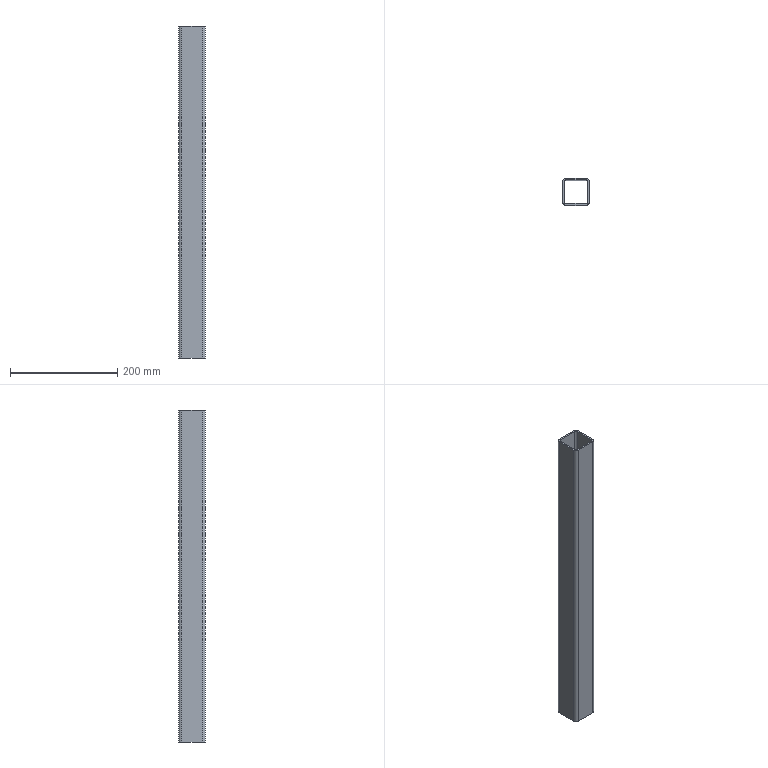Part | SolidWorks | 1 solid | 18 faces | box 50 x 50 x 620 mm | volume 335310 mm3 | plane 10 | cylinder 8 | commonest cylinder face diameters 6 x4 12 x4
STEP:
#1=CARTESIAN_POINT('',(19.,25.,310.));
#2=VERTEX_POINT('',#1);
#3=CARTESIAN_POINT('',(25.,19.,310.));
#4=VERTEX_POINT('',#3);
#5=CARTESIAN_POINT('',(19.,19.,310.));
#6=DIRECTION('',(0.,0.,-1.));
#7=DIRECTION('',(-1.,0.,0.));
#8=AXIS2_PLACEMENT_3D('',#5,#6,#7);
#9=CIRCLE('',#8,6.);
#10=EDGE_CURVE('',#2,#4,#9,.T.);
#11=ORIENTED_EDGE('',*,*,#10,.T.);
#12=CARTESIAN_POINT('',(25.,19.,-310.));
#13=VERTEX_POINT('',#12);
#14=CARTESIAN_POINT('',(25.,19.,-310.));
#15=DIRECTION('',(0.,0.,1.));
#16=VECTOR('',#15,1000.);
#17=LINE('',#14,#16);
#18=EDGE_CURVE('',#13,#4,#17,.T.);
#19=ORIENTED_EDGE('',*,*,#18,.F.);
#20=CARTESIAN_POINT('',(19.,25.,-310.));
#21=VERTEX_POINT('',#20);
#22=CARTESIAN_POINT('',(19.,19.,-310.));
#23=DIRECTION('',(0.,0.,-1.));
#24=DIRECTION('',(-1.,0.,0.));
#25=AXIS2_PLACEMENT_3D('',#22,#23,#24);
#26=CIRCLE('',#25,6.);
#27=EDGE_CURVE('',#21,#13,#26,.T.);
#28=ORIENTED_EDGE('',*,*,#27,.F.);
#29=CARTESIAN_POINT('',(19.,25.,-310.));
#30=DIRECTION('',(0.,0.,1.));
#31=VECTOR('',#30,1000.);
#32=LINE('',#29,#31);
#33=EDGE_CURVE('',#21,#2,#32,.T.);
#34=ORIENTED_EDGE('',*,*,#33,.T.);
#35=EDGE_LOOP('',(#11,#19,#28,#34));
#36=FACE_OUTER_BOUND('',#35,.T.);
#37=CARTESIAN_POINT('',(19.,19.,-310.));
#38=DIRECTION('',(0.,0.,1.));
#39=DIRECTION('',(1.,0.,0.));
#40=AXIS2_PLACEMENT_3D('',#37,#38,#39);
#41=CYLINDRICAL_SURFACE('',#40,6.);
#42=ADVANCED_FACE('',(#36),#41,.T.);
#43=CARTESIAN_POINT('',(25.,-19.,310.));
#44=VERTEX_POINT('',#43);
#45=CARTESIAN_POINT('',(25.,19.,310.));
#46=DIRECTION('',(0.,-1.,0.));
#47=VECTOR('',#46,1000.);
#48=LINE('',#45,#47);
#49=EDGE_CURVE('',#4,#44,#48,.T.);
#50=ORIENTED_EDGE('',*,*,#49,.T.);
#51=CARTESIAN_POINT('',(25.,-19.,-310.));
#52=VERTEX_POINT('',#51);
#53=CARTESIAN_POINT('',(25.,-19.,-310.));
#54=DIRECTION('',(0.,0.,1.));
#55=VECTOR('',#54,1000.);
#56=LINE('',#53,#55);
#57=EDGE_CURVE('',#52,#44,#56,.T.);
#58=ORIENTED_EDGE('',*,*,#57,.F.);
#59=CARTESIAN_POINT('',(25.,19.,-310.));
#60=DIRECTION('',(0.,-1.,0.));
#61=VECTOR('',#60,1000.);
#62=LINE('',#59,#61);
#63=EDGE_CURVE('',#13,#52,#62,.T.);
#64=ORIENTED_EDGE('',*,*,#63,.F.);
#65=ORIENTED_EDGE('',*,*,#18,.T.);
#66=EDGE_LOOP('',(#50,#58,#64,#65));
#67=FACE_OUTER_BOUND('',#66,.T.);
#68=CARTESIAN_POINT('',(25.,19.,-310.));
#69=DIRECTION('',(-1.,0.,0.));
#70=DIRECTION('',(0.,0.,1.));
#71=AXIS2_PLACEMENT_3D('',#68,#69,#70);
#72=PLANE('',#71);
#73=ADVANCED_FACE('',(#67),#72,.F.);
#74=CARTESIAN_POINT('',(19.,-25.,310.));
#75=VERTEX_POINT('',#74);
#76=CARTESIAN_POINT('',(19.,-19.,310.));
#77=DIRECTION('',(0.,0.,-1.));
#78=DIRECTION('',(-1.,0.,0.));
#79=AXIS2_PLACEMENT_3D('',#76,#77,#78);
#80=CIRCLE('',#79,6.);
#81=EDGE_CURVE('',#44,#75,#80,.T.);
#82=ORIENTED_EDGE('',*,*,#81,.T.);
#83=CARTESIAN_POINT('',(19.,-25.,-310.));
#84=VERTEX_POINT('',#83);
#85=CARTESIAN_POINT('',(19.,-25.,-310.));
#86=DIRECTION('',(0.,0.,1.));
#87=VECTOR('',#86,1000.);
#88=LINE('',#85,#87);
#89=EDGE_CURVE('',#84,#75,#88,.T.);
#90=ORIENTED_EDGE('',*,*,#89,.F.);
#91=CARTESIAN_POINT('',(19.,-19.,-310.));
#92=DIRECTION('',(0.,0.,-1.));
#93=DIRECTION('',(-1.,0.,0.));
#94=AXIS2_PLACEMENT_3D('',#91,#92,#93);
#95=CIRCLE('',#94,6.);
#96=EDGE_CURVE('',#52,#84,#95,.T.);
#97=ORIENTED_EDGE('',*,*,#96,.F.);
#98=ORIENTED_EDGE('',*,*,#57,.T.);
#99=EDGE_LOOP('',(#82,#90,#97,#98));
#100=FACE_OUTER_BOUND('',#99,.T.);
#101=CARTESIAN_POINT('',(19.,-19.,-310.));
#102=DIRECTION('',(0.,0.,1.));
#103=DIRECTION('',(1.,0.,0.));
#104=AXIS2_PLACEMENT_3D('',#101,#102,#103);
#105=CYLINDRICAL_SURFACE('',#104,6.);
#106=ADVANCED_FACE('',(#100),#105,.T.);
#107=CARTESIAN_POINT('',(-19.,-25.,310.));
#108=VERTEX_POINT('',#107);
#109=CARTESIAN_POINT('',(-19.,-25.,310.));
#110=DIRECTION('',(-1.,0.,0.));
#111=VECTOR('',#110,1000.);
#112=LINE('',#109,#111);
#113=EDGE_CURVE('',#75,#108,#112,.T.);
#114=ORIENTED_EDGE('',*,*,#113,.T.);
#115=CARTESIAN_POINT('',(-19.,-25.,-310.));
#116=VERTEX_POINT('',#115);
#117=CARTESIAN_POINT('',(-19.,-25.,-310.));
#118=DIRECTION('',(0.,0.,1.));
#119=VECTOR('',#118,1000.);
#120=LINE('',#117,#119);
#121=EDGE_CURVE('',#116,#108,#120,.T.);
#122=ORIENTED_EDGE('',*,*,#121,.F.);
#123=CARTESIAN_POINT('',(-19.,-25.,-310.));
#124=DIRECTION('',(-1.,0.,0.));
#125=VECTOR('',#124,1000.);
#126=LINE('',#123,#125);
#127=EDGE_CURVE('',#84,#116,#126,.T.);
#128=ORIENTED_EDGE('',*,*,#127,.F.);
#129=ORIENTED_EDGE('',*,*,#89,.T.);
#130=EDGE_LOOP('',(#114,#122,#128,#129));
#131=FACE_OUTER_BOUND('',#130,.T.);
#132=CARTESIAN_POINT('',(-19.,-25.,-310.));
#133=DIRECTION('',(0.,1.,0.));
#134=DIRECTION('',(0.,0.,1.));
#135=AXIS2_PLACEMENT_3D('',#132,#133,#134);
#136=PLANE('',#135);
#137=ADVANCED_FACE('',(#131),#136,.F.);
#138=CARTESIAN_POINT('',(-25.,-19.,310.));
#139=VERTEX_POINT('',#138);
#140=CARTESIAN_POINT('',(-19.,-19.,310.));
#141=DIRECTION('',(0.,0.,-1.));
#142=DIRECTION('',(-1.,0.,0.));
#143=AXIS2_PLACEMENT_3D('',#140,#141,#142);
#144=CIRCLE('',#143,6.);
#145=EDGE_CURVE('',#108,#139,#144,.T.);
#146=ORIENTED_EDGE('',*,*,#145,.T.);
#147=CARTESIAN_POINT('',(-25.,-19.,-310.));
#148=VERTEX_POINT('',#147);
#149=CARTESIAN_POINT('',(-25.,-19.,-310.));
#150=DIRECTION('',(0.,0.,1.));
#151=VECTOR('',#150,1000.);
#152=LINE('',#149,#151);
#153=EDGE_CURVE('',#148,#139,#152,.T.);
#154=ORIENTED_EDGE('',*,*,#153,.F.);
#155=CARTESIAN_POINT('',(-19.,-19.,-310.));
#156=DIRECTION('',(0.,0.,-1.));
#157=DIRECTION('',(-1.,0.,0.));
#158=AXIS2_PLACEMENT_3D('',#155,#156,#157);
#159=CIRCLE('',#158,6.);
#160=EDGE_CURVE('',#116,#148,#159,.T.);
#161=ORIENTED_EDGE('',*,*,#160,.F.);
#162=ORIENTED_EDGE('',*,*,#121,.T.);
#163=EDGE_LOOP('',(#146,#154,#161,#162));
#164=FACE_OUTER_BOUND('',#163,.T.);
#165=CARTESIAN_POINT('',(-19.,-19.,-310.));
#166=DIRECTION('',(0.,0.,1.));
#167=DIRECTION('',(1.,0.,0.));
#168=AXIS2_PLACEMENT_3D('',#165,#166,#167);
#169=CYLINDRICAL_SURFACE('',#168,6.);
#170=ADVANCED_FACE('',(#164),#169,.T.);
#171=CARTESIAN_POINT('',(-25.,19.,310.));
#172=VERTEX_POINT('',#171);
#173=CARTESIAN_POINT('',(-25.,-19.,310.));
#174=DIRECTION('',(0.,1.,0.));
#175=VECTOR('',#174,1000.);
#176=LINE('',#173,#175);
#177=EDGE_CURVE('',#139,#172,#176,.T.);
#178=ORIENTED_EDGE('',*,*,#177,.T.);
#179=CARTESIAN_POINT('',(-25.,19.,-310.));
#180=VERTEX_POINT('',#179);
#181=CARTESIAN_POINT('',(-25.,19.,-310.));
#182=DIRECTION('',(0.,0.,1.));
#183=VECTOR('',#182,1000.);
#184=LINE('',#181,#183);
#185=EDGE_CURVE('',#180,#172,#184,.T.);
#186=ORIENTED_EDGE('',*,*,#185,.F.);
#187=CARTESIAN_POINT('',(-25.,-19.,-310.));
#188=DIRECTION('',(0.,1.,0.));
#189=VECTOR('',#188,1000.);
#190=LINE('',#187,#189);
#191=EDGE_CURVE('',#148,#180,#190,.T.);
#192=ORIENTED_EDGE('',*,*,#191,.F.);
#193=ORIENTED_EDGE('',*,*,#153,.T.);
#194=EDGE_LOOP('',(#178,#186,#192,#193));
#195=FACE_OUTER_BOUND('',#194,.T.);
#196=CARTESIAN_POINT('',(-25.,-19.,-310.));
#197=DIRECTION('',(1.,0.,0.));
#198=DIRECTION('',(0.,0.,-1.));
#199=AXIS2_PLACEMENT_3D('',#196,#197,#198);
#200=PLANE('',#199);
#201=ADVANCED_FACE('',(#195),#200,.F.);
#202=CARTESIAN_POINT('',(-19.,25.,310.));
#203=VERTEX_POINT('',#202);
#204=CARTESIAN_POINT('',(-19.,19.,310.));
#205=DIRECTION('',(0.,0.,-1.));
#206=DIRECTION('',(-1.,0.,0.));
#207=AXIS2_PLACEMENT_3D('',#204,#205,#206);
#208=CIRCLE('',#207,6.);
#209=EDGE_CURVE('',#172,#203,#208,.T.);
#210=ORIENTED_EDGE('',*,*,#209,.T.);
#211=CARTESIAN_POINT('',(-19.,25.,-310.));
#212=VERTEX_POINT('',#211);
#213=CARTESIAN_POINT('',(-19.,25.,-310.));
#214=DIRECTION('',(0.,0.,1.));
#215=VECTOR('',#214,1000.);
#216=LINE('',#213,#215);
#217=EDGE_CURVE('',#212,#203,#216,.T.);
#218=ORIENTED_EDGE('',*,*,#217,.F.);
#219=CARTESIAN_POINT('',(-19.,19.,-310.));
#220=DIRECTION('',(0.,0.,-1.));
#221=DIRECTION('',(-1.,0.,0.));
#222=AXIS2_PLACEMENT_3D('',#219,#220,#221);
#223=CIRCLE('',#222,6.);
#224=EDGE_CURVE('',#180,#212,#223,.T.);
#225=ORIENTED_EDGE('',*,*,#224,.F.);
#226=ORIENTED_EDGE('',*,*,#185,.T.);
#227=EDGE_LOOP('',(#210,#218,#225,#226));
#228=FACE_OUTER_BOUND('',#227,.T.);
#229=CARTESIAN_POINT('',(-19.,19.,-310.));
#230=DIRECTION('',(0.,0.,1.));
#231=DIRECTION('',(1.,0.,0.));
#232=AXIS2_PLACEMENT_3D('',#229,#230,#231);
#233=CYLINDRICAL_SURFACE('',#232,6.);
#234=ADVANCED_FACE('',(#228),#233,.T.);
#235=CARTESIAN_POINT('',(22.,-19.,310.));
#236=VERTEX_POINT('',#235);
#237=CARTESIAN_POINT('',(19.,-22.,310.));
#238=VERTEX_POINT('',#237);
#239=CARTESIAN_POINT('',(19.,-19.,310.));
#240=DIRECTION('',(0.,0.,-1.));
#241=DIRECTION('',(-1.,0.,0.));
#242=AXIS2_PLACEMENT_3D('',#239,#240,#241);
#243=CIRCLE('',#242,3.);
#244=EDGE_CURVE('',#236,#238,#243,.T.);
#245=ORIENTED_EDGE('',*,*,#244,.F.);
#246=CARTESIAN_POINT('',(22.,-19.,-310.));
#247=VERTEX_POINT('',#246);
#248=CARTESIAN_POINT('',(22.,-19.,-310.));
#249=DIRECTION('',(0.,0.,1.));
#250=VECTOR('',#249,1000.);
#251=LINE('',#248,#250);
#252=EDGE_CURVE('',#247,#236,#251,.T.);
#253=ORIENTED_EDGE('',*,*,#252,.F.);
#254=CARTESIAN_POINT('',(19.,-22.,-310.));
#255=VERTEX_POINT('',#254);
#256=CARTESIAN_POINT('',(19.,-19.,-310.));
#257=DIRECTION('',(0.,0.,-1.));
#258=DIRECTION('',(-1.,0.,0.));
#259=AXIS2_PLACEMENT_3D('',#256,#257,#258);
#260=CIRCLE('',#259,3.);
#261=EDGE_CURVE('',#247,#255,#260,.T.);
#262=ORIENTED_EDGE('',*,*,#261,.T.);
#263=CARTESIAN_POINT('',(19.,-22.,-310.));
#264=DIRECTION('',(0.,0.,1.));
#265=VECTOR('',#264,1000.);
#266=LINE('',#263,#265);
#267=EDGE_CURVE('',#255,#238,#266,.T.);
#268=ORIENTED_EDGE('',*,*,#267,.T.);
#269=EDGE_LOOP('',(#245,#253,#262,#268));
#270=FACE_OUTER_BOUND('',#269,.T.);
#271=CARTESIAN_POINT('',(19.,-19.,-310.));
#272=DIRECTION('',(0.,0.,1.));
#273=DIRECTION('',(1.,0.,0.));
#274=AXIS2_PLACEMENT_3D('',#271,#272,#273);
#275=CYLINDRICAL_SURFACE('',#274,3.);
#276=ADVANCED_FACE('',(#270),#275,.F.);
#277=CARTESIAN_POINT('',(22.,19.,310.));
#278=VERTEX_POINT('',#277);
#279=CARTESIAN_POINT('',(22.,19.,310.));
#280=DIRECTION('',(0.,-1.,0.));
#281=VECTOR('',#280,1000.);
#282=LINE('',#279,#281);
#283=EDGE_CURVE('',#278,#236,#282,.T.);
#284=ORIENTED_EDGE('',*,*,#283,.F.);
#285=CARTESIAN_POINT('',(22.,19.,-310.));
#286=VERTEX_POINT('',#285);
#287=CARTESIAN_POINT('',(22.,19.,-310.));
#288=DIRECTION('',(0.,0.,1.));
#289=VECTOR('',#288,1000.);
#290=LINE('',#287,#289);
#291=EDGE_CURVE('',#286,#278,#290,.T.);
#292=ORIENTED_EDGE('',*,*,#291,.F.);
#293=CARTESIAN_POINT('',(22.,19.,-310.));
#294=DIRECTION('',(0.,-1.,0.));
#295=VECTOR('',#294,1000.);
#296=LINE('',#293,#295);
#297=EDGE_CURVE('',#286,#247,#296,.T.);
#298=ORIENTED_EDGE('',*,*,#297,.T.);
#299=ORIENTED_EDGE('',*,*,#252,.T.);
#300=EDGE_LOOP('',(#284,#292,#298,#299));
#301=FACE_OUTER_BOUND('',#300,.T.);
#302=CARTESIAN_POINT('',(22.,19.,-310.));
#303=DIRECTION('',(-1.,0.,0.));
#304=DIRECTION('',(0.,0.,1.));
#305=AXIS2_PLACEMENT_3D('',#302,#303,#304);
#306=PLANE('',#305);
#307=ADVANCED_FACE('',(#301),#306,.T.);
#308=CARTESIAN_POINT('',(19.,22.,310.));
#309=VERTEX_POINT('',#308);
#310=CARTESIAN_POINT('',(19.,19.,310.));
#311=DIRECTION('',(0.,0.,-1.));
#312=DIRECTION('',(-1.,0.,0.));
#313=AXIS2_PLACEMENT_3D('',#310,#311,#312);
#314=CIRCLE('',#313,3.);
#315=EDGE_CURVE('',#309,#278,#314,.T.);
#316=ORIENTED_EDGE('',*,*,#315,.F.);
#317=CARTESIAN_POINT('',(19.,22.,-310.));
#318=VERTEX_POINT('',#317);
#319=CARTESIAN_POINT('',(19.,22.,-310.));
#320=DIRECTION('',(0.,0.,1.));
#321=VECTOR('',#320,1000.);
#322=LINE('',#319,#321);
#323=EDGE_CURVE('',#318,#309,#322,.T.);
#324=ORIENTED_EDGE('',*,*,#323,.F.);
#325=CARTESIAN_POINT('',(19.,19.,-310.));
#326=DIRECTION('',(0.,0.,-1.));
#327=DIRECTION('',(-1.,0.,0.));
#328=AXIS2_PLACEMENT_3D('',#325,#326,#327);
#329=CIRCLE('',#328,3.);
#330=EDGE_CURVE('',#318,#286,#329,.T.);
#331=ORIENTED_EDGE('',*,*,#330,.T.);
#332=ORIENTED_EDGE('',*,*,#291,.T.);
#333=EDGE_LOOP('',(#316,#324,#331,#332));
#334=FACE_OUTER_BOUND('',#333,.T.);
#335=CARTESIAN_POINT('',(19.,19.,-310.));
#336=DIRECTION('',(0.,0.,1.));
#337=DIRECTION('',(1.,0.,0.));
#338=AXIS2_PLACEMENT_3D('',#335,#336,#337);
#339=CYLINDRICAL_SURFACE('',#338,3.);
#340=ADVANCED_FACE('',(#334),#339,.F.);
#341=CARTESIAN_POINT('',(-19.,22.,310.));
#342=VERTEX_POINT('',#341);
#343=CARTESIAN_POINT('',(19.,22.,310.));
#344=DIRECTION('',(1.,0.,0.));
#345=VECTOR('',#344,1000.);
#346=LINE('',#343,#345);
#347=EDGE_CURVE('',#342,#309,#346,.T.);
#348=ORIENTED_EDGE('',*,*,#347,.F.);
#349=CARTESIAN_POINT('',(-19.,22.,-310.));
#350=VERTEX_POINT('',#349);
#351=CARTESIAN_POINT('',(-19.,22.,-310.));
#352=DIRECTION('',(0.,0.,1.));
#353=VECTOR('',#352,1000.);
#354=LINE('',#351,#353);
#355=EDGE_CURVE('',#350,#342,#354,.T.);
#356=ORIENTED_EDGE('',*,*,#355,.F.);
#357=CARTESIAN_POINT('',(19.,22.,-310.));
#358=DIRECTION('',(1.,0.,0.));
#359=VECTOR('',#358,1000.);
#360=LINE('',#357,#359);
#361=EDGE_CURVE('',#350,#318,#360,.T.);
#362=ORIENTED_EDGE('',*,*,#361,.T.);
#363=ORIENTED_EDGE('',*,*,#323,.T.);
#364=EDGE_LOOP('',(#348,#356,#362,#363));
#365=FACE_OUTER_BOUND('',#364,.T.);
#366=CARTESIAN_POINT('',(19.,22.,-310.));
#367=DIRECTION('',(0.,-1.,0.));
#368=DIRECTION('',(0.,0.,-1.));
#369=AXIS2_PLACEMENT_3D('',#366,#367,#368);
#370=PLANE('',#369);
#371=ADVANCED_FACE('',(#365),#370,.T.);
#372=CARTESIAN_POINT('',(-22.,19.,310.));
#373=VERTEX_POINT('',#372);
#374=CARTESIAN_POINT('',(-19.,19.,310.));
#375=DIRECTION('',(0.,0.,-1.));
#376=DIRECTION('',(-1.,0.,0.));
#377=AXIS2_PLACEMENT_3D('',#374,#375,#376);
#378=CIRCLE('',#377,3.);
#379=EDGE_CURVE('',#373,#342,#378,.T.);
#380=ORIENTED_EDGE('',*,*,#379,.F.);
#381=CARTESIAN_POINT('',(-22.,19.,-310.));
#382=VERTEX_POINT('',#381);
#383=CARTESIAN_POINT('',(-22.,19.,-310.));
#384=DIRECTION('',(0.,0.,1.));
#385=VECTOR('',#384,1000.);
#386=LINE('',#383,#385);
#387=EDGE_CURVE('',#382,#373,#386,.T.);
#388=ORIENTED_EDGE('',*,*,#387,.F.);
#389=CARTESIAN_POINT('',(-19.,19.,-310.));
#390=DIRECTION('',(0.,0.,-1.));
#391=DIRECTION('',(-1.,0.,0.));
#392=AXIS2_PLACEMENT_3D('',#389,#390,#391);
#393=CIRCLE('',#392,3.);
#394=EDGE_CURVE('',#382,#350,#393,.T.);
#395=ORIENTED_EDGE('',*,*,#394,.T.);
#396=ORIENTED_EDGE('',*,*,#355,.T.);
#397=EDGE_LOOP('',(#380,#388,#395,#396));
#398=FACE_OUTER_BOUND('',#397,.T.);
#399=CARTESIAN_POINT('',(-19.,19.,-310.));
#400=DIRECTION('',(0.,0.,1.));
#401=DIRECTION('',(1.,0.,0.));
#402=AXIS2_PLACEMENT_3D('',#399,#400,#401);
#403=CYLINDRICAL_SURFACE('',#402,3.);
#404=ADVANCED_FACE('',(#398),#403,.F.);
#405=CARTESIAN_POINT('',(-22.,-19.,310.));
#406=VERTEX_POINT('',#405);
#407=CARTESIAN_POINT('',(-22.,-19.,310.));
#408=DIRECTION('',(0.,1.,0.));
#409=VECTOR('',#408,1000.);
#410=LINE('',#407,#409);
#411=EDGE_CURVE('',#406,#373,#410,.T.);
#412=ORIENTED_EDGE('',*,*,#411,.F.);
#413=CARTESIAN_POINT('',(-22.,-19.,-310.));
#414=VERTEX_POINT('',#413);
#415=CARTESIAN_POINT('',(-22.,-19.,-310.));
#416=DIRECTION('',(0.,0.,1.));
#417=VECTOR('',#416,1000.);
#418=LINE('',#415,#417);
#419=EDGE_CURVE('',#414,#406,#418,.T.);
#420=ORIENTED_EDGE('',*,*,#419,.F.);
#421=CARTESIAN_POINT('',(-22.,-19.,-310.));
#422=DIRECTION('',(0.,1.,0.));
#423=VECTOR('',#422,1000.);
#424=LINE('',#421,#423);
#425=EDGE_CURVE('',#414,#382,#424,.T.);
#426=ORIENTED_EDGE('',*,*,#425,.T.);
#427=ORIENTED_EDGE('',*,*,#387,.T.);
#428=EDGE_LOOP('',(#412,#420,#426,#427));
#429=FACE_OUTER_BOUND('',#428,.T.);
#430=CARTESIAN_POINT('',(-22.,-19.,-310.));
#431=DIRECTION('',(1.,0.,0.));
#432=DIRECTION('',(0.,0.,-1.));
#433=AXIS2_PLACEMENT_3D('',#430,#431,#432);
#434=PLANE('',#433);
#435=ADVANCED_FACE('',(#429),#434,.T.);
#436=CARTESIAN_POINT('',(-19.,-22.,310.));
#437=VERTEX_POINT('',#436);
#438=CARTESIAN_POINT('',(-19.,-19.,310.));
#439=DIRECTION('',(0.,0.,-1.));
#440=DIRECTION('',(-1.,0.,0.));
#441=AXIS2_PLACEMENT_3D('',#438,#439,#440);
#442=CIRCLE('',#441,3.);
#443=EDGE_CURVE('',#437,#406,#442,.T.);
#444=ORIENTED_EDGE('',*,*,#443,.F.);
#445=CARTESIAN_POINT('',(-19.,-22.,-310.));
#446=VERTEX_POINT('',#445);
#447=CARTESIAN_POINT('',(-19.,-22.,-310.));
#448=DIRECTION('',(0.,0.,1.));
#449=VECTOR('',#448,1000.);
#450=LINE('',#447,#449);
#451=EDGE_CURVE('',#446,#437,#450,.T.);
#452=ORIENTED_EDGE('',*,*,#451,.F.);
#453=CARTESIAN_POINT('',(-19.,-19.,-310.));
#454=DIRECTION('',(0.,0.,-1.));
#455=DIRECTION('',(-1.,0.,0.));
#456=AXIS2_PLACEMENT_3D('',#453,#454,#455);
#457=CIRCLE('',#456,3.);
#458=EDGE_CURVE('',#446,#414,#457,.T.);
#459=ORIENTED_EDGE('',*,*,#458,.T.);
#460=ORIENTED_EDGE('',*,*,#419,.T.);
#461=EDGE_LOOP('',(#444,#452,#459,#460));
#462=FACE_OUTER_BOUND('',#461,.T.);
#463=CARTESIAN_POINT('',(-19.,-19.,-310.));
#464=DIRECTION('',(0.,0.,1.));
#465=DIRECTION('',(1.,0.,0.));
#466=AXIS2_PLACEMENT_3D('',#463,#464,#465);
#467=CYLINDRICAL_SURFACE('',#466,3.);
#468=ADVANCED_FACE('',(#462),#467,.F.);
#469=CARTESIAN_POINT('',(-19.,-22.,310.));
#470=DIRECTION('',(-1.,0.,0.));
#471=VECTOR('',#470,1000.);
#472=LINE('',#469,#471);
#473=EDGE_CURVE('',#238,#437,#472,.T.);
#474=ORIENTED_EDGE('',*,*,#473,.F.);
#475=ORIENTED_EDGE('',*,*,#267,.F.);
#476=CARTESIAN_POINT('',(-19.,-22.,-310.));
#477=DIRECTION('',(-1.,0.,0.));
#478=VECTOR('',#477,1000.);
#479=LINE('',#476,#478);
#480=EDGE_CURVE('',#255,#446,#479,.T.);
#481=ORIENTED_EDGE('',*,*,#480,.T.);
#482=ORIENTED_EDGE('',*,*,#451,.T.);
#483=EDGE_LOOP('',(#474,#475,#481,#482));
#484=FACE_OUTER_BOUND('',#483,.T.);
#485=CARTESIAN_POINT('',(-19.,-22.,-310.));
#486=DIRECTION('',(0.,1.,0.));
#487=DIRECTION('',(0.,0.,1.));
#488=AXIS2_PLACEMENT_3D('',#485,#486,#487);
#489=PLANE('',#488);
#490=ADVANCED_FACE('',(#484),#489,.T.);
#491=CARTESIAN_POINT('',(19.,25.,310.));
#492=DIRECTION('',(1.,0.,0.));
#493=VECTOR('',#492,1000.);
#494=LINE('',#491,#493);
#495=EDGE_CURVE('',#203,#2,#494,.T.);
#496=ORIENTED_EDGE('',*,*,#495,.T.);
#497=ORIENTED_EDGE('',*,*,#33,.F.);
#498=CARTESIAN_POINT('',(19.,25.,-310.));
#499=DIRECTION('',(1.,0.,0.));
#500=VECTOR('',#499,1000.);
#501=LINE('',#498,#500);
#502=EDGE_CURVE('',#212,#21,#501,.T.);
#503=ORIENTED_EDGE('',*,*,#502,.F.);
#504=ORIENTED_EDGE('',*,*,#217,.T.);
#505=EDGE_LOOP('',(#496,#497,#503,#504));
#506=FACE_OUTER_BOUND('',#505,.T.);
#507=CARTESIAN_POINT('',(19.,25.,-310.));
#508=DIRECTION('',(0.,-1.,0.));
#509=DIRECTION('',(0.,0.,-1.));
#510=AXIS2_PLACEMENT_3D('',#507,#508,#509);
#511=PLANE('',#510);
#512=ADVANCED_FACE('',(#506),#511,.F.);
#513=ORIENTED_EDGE('',*,*,#261,.F.);
#514=ORIENTED_EDGE('',*,*,#297,.F.);
#515=ORIENTED_EDGE('',*,*,#330,.F.);
#516=ORIENTED_EDGE('',*,*,#361,.F.);
#517=ORIENTED_EDGE('',*,*,#394,.F.);
#518=ORIENTED_EDGE('',*,*,#425,.F.);
#519=ORIENTED_EDGE('',*,*,#458,.F.);
#520=ORIENTED_EDGE('',*,*,#480,.F.);
#521=EDGE_LOOP('',(#513,#514,#515,#516,#517,#518,#519,#520));
#522=FACE_BOUND('',#521,.T.);
#523=ORIENTED_EDGE('',*,*,#27,.T.);
#524=ORIENTED_EDGE('',*,*,#63,.T.);
#525=ORIENTED_EDGE('',*,*,#96,.T.);
#526=ORIENTED_EDGE('',*,*,#127,.T.);
#527=ORIENTED_EDGE('',*,*,#160,.T.);
#528=ORIENTED_EDGE('',*,*,#191,.T.);
#529=ORIENTED_EDGE('',*,*,#224,.T.);
#530=ORIENTED_EDGE('',*,*,#502,.T.);
#531=EDGE_LOOP('',(#523,#524,#525,#526,#527,#528,#529,#530));
#532=FACE_OUTER_BOUND('',#531,.T.);
#533=CARTESIAN_POINT('',(19.,19.,-310.));
#534=DIRECTION('',(0.,0.,-1.));
#535=DIRECTION('',(-1.,0.,0.));
#536=AXIS2_PLACEMENT_3D('',#533,#534,#535);
#537=PLANE('',#536);
#538=ADVANCED_FACE('',(#522,#532),#537,.T.);
#539=ORIENTED_EDGE('',*,*,#244,.T.);
#540=ORIENTED_EDGE('',*,*,#473,.T.);
#541=ORIENTED_EDGE('',*,*,#443,.T.);
#542=ORIENTED_EDGE('',*,*,#411,.T.);
#543=ORIENTED_EDGE('',*,*,#379,.T.);
#544=ORIENTED_EDGE('',*,*,#347,.T.);
#545=ORIENTED_EDGE('',*,*,#315,.T.);
#546=ORIENTED_EDGE('',*,*,#283,.T.);
#547=EDGE_LOOP('',(#539,#540,#541,#542,#543,#544,#545,#546));
#548=FACE_BOUND('',#547,.T.);
#549=ORIENTED_EDGE('',*,*,#10,.F.);
#550=ORIENTED_EDGE('',*,*,#495,.F.);
#551=ORIENTED_EDGE('',*,*,#209,.F.);
#552=ORIENTED_EDGE('',*,*,#177,.F.);
#553=ORIENTED_EDGE('',*,*,#145,.F.);
#554=ORIENTED_EDGE('',*,*,#113,.F.);
#555=ORIENTED_EDGE('',*,*,#81,.F.);
#556=ORIENTED_EDGE('',*,*,#49,.F.);
#557=EDGE_LOOP('',(#549,#550,#551,#552,#553,#554,#555,#556));
#558=FACE_OUTER_BOUND('',#557,.T.);
#559=CARTESIAN_POINT('',(19.,19.,310.));
#560=DIRECTION('',(0.,0.,-1.));
#561=DIRECTION('',(-1.,0.,0.));
#562=AXIS2_PLACEMENT_3D('',#559,#560,#561);
#563=PLANE('',#562);
#564=ADVANCED_FACE('',(#548,#558),#563,.F.);
#565=CLOSED_SHELL('',(#42,#73,#106,#137,#170,#201,#234,#276,#307,#340,#371,#404,#435,#468,#490,#512,#538,#564));
#566=MANIFOLD_SOLID_BREP('',#565);
#567=CARTESIAN_POINT('',(0.,0.,0.));
#568=DIRECTION('',(0.,0.,1.));
#569=DIRECTION('',(1.,0.,0.));
#570=AXIS2_PLACEMENT_3D('',#567,#568,#569);
#571=(LENGTH_UNIT()NAMED_UNIT(*)SI_UNIT(.MILLI.,.METRE.));
#572=UNCERTAINTY_MEASURE_WITH_UNIT(LENGTH_MEASURE(0.00001),#571,'','');
#573=(NAMED_UNIT(*)PLANE_ANGLE_UNIT()SI_UNIT($,.RADIAN.));
#574=(NAMED_UNIT(*)SI_UNIT($,.STERADIAN.)SOLID_ANGLE_UNIT());
#575=(GEOMETRIC_REPRESENTATION_CONTEXT(3)GLOBAL_UNCERTAINTY_ASSIGNED_CONTEXT((#572))GLOBAL_UNIT_ASSIGNED_CONTEXT((#571,#573,#574))REPRESENTATION_CONTEXT('',''));
#576=ADVANCED_BREP_SHAPE_REPRESENTATION('',(#566,#570),#575);